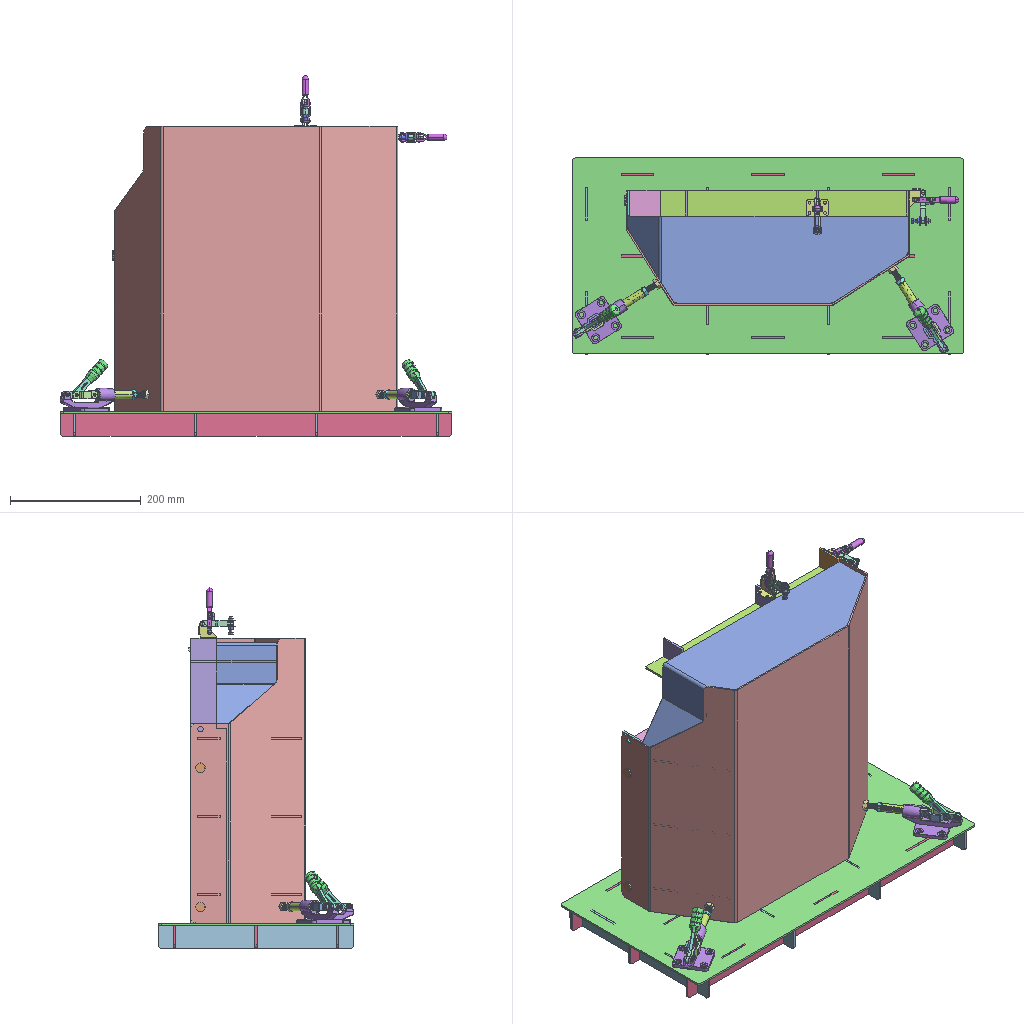Assembly | SolidWorks | 13 different items | 24 placed | box 600 x 300 x 552 mm
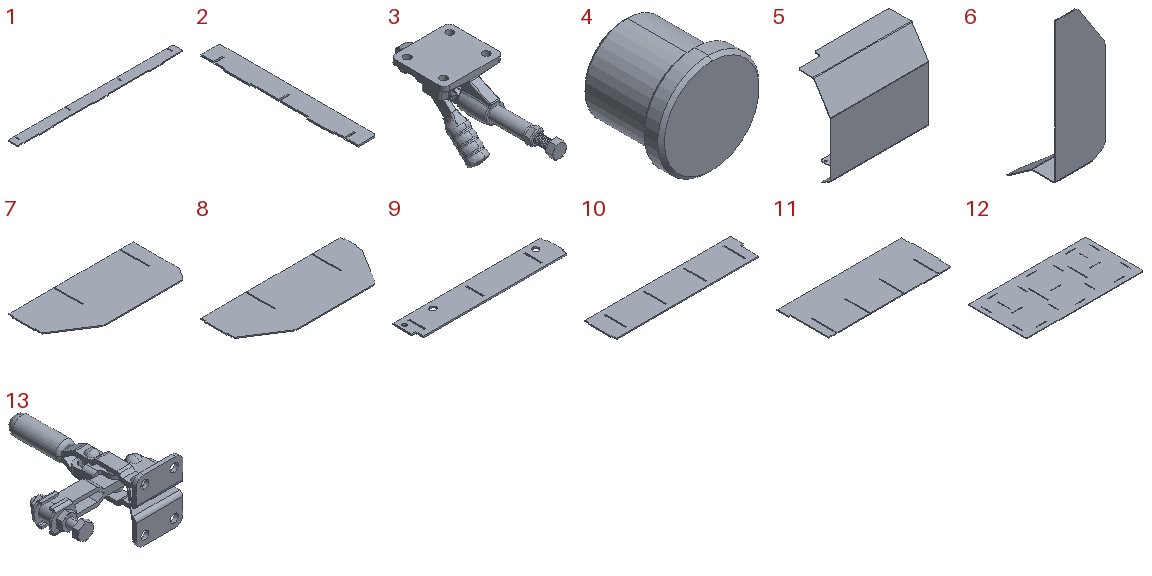Parts list (item | quantity | size | volume | features):
1 | x3 | 600 x 38 x 3.2 mm | 67879 mm3 | features FlatPattern 1, SMBaseFlange 1, SheetMetal 1
2 | x4 | 38 x 300 x 3.2 mm | 33980 mm3 | features FlatPattern 1, SMBaseFlange 1, SheetMetal 1
3 | x2 | 57.2 x 153.749 x 79.304 mm | 52807 mm3 | features BaseBody 11
4 | x2 | 15 x 13 x 15 mm | 1741 mm3 | features Chamfer 1, Revolution 1
5 | x1 | 436 x 176 x 434 mm | 633093 mm3 | features ICE 3, Fillet 1, FlatPattern 1, SMBaseFlange 1, SheetMetal 1
6 | x1 | 134 x 132 x 429.026 mm | 130634 mm3 | features Chamfer 1, FlatPattern 1, ICE 1, SMBaseFlange 1, SheetMetal 1
7 | x1 | 379.5 x 173.7 x 3.2 mm | 193629 mm3 | features FlatPattern 1, SMBaseFlange 1, SheetMetal 1
8 | x3 | 429 x 173.7 x 3.2 mm | 209173 mm3 | features FlatPattern 1, SMBaseFlange 1, SheetMetal 1
9 | x1 | 309 x 55 x 3.2 mm | 51735 mm3 | features FlatPattern 1, SMBaseFlange 1, SheetMetal 1
10 | x1 | 439 x 95 x 3.2 mm | 129037 mm3 | features FlatPattern 1, SMBaseFlange 1, SheetMetal 1
11 | x2 | 439 x 173.7 x 3.2 mm | 236184 mm3 | features FlatPattern 1, SMBaseFlange 1, SheetMetal 1
12 | x1 | 600 x 300 x 3.2 mm | 564155 mm3 | features FlatPattern 1, SMBaseFlange 1, SheetMetal 1
13 | x2 | 56.45 x 77.62 x 33.3 mm | 10418 mm3 | features BaseBody 5
Mates (type | each side: item.copy, entity, surface, feature):
DistanceDim | 6.1 face plane Base-Flange1 | 5.1 face plane Base-Flange1
Coincident | 5.1 face plane Base-Flange1 | 6.1 face plane Base-Flange1 | 2 times
InPlace | 7.1 plane | assembly plane
InPlace | 8.1 plane | assembly plane
InPlace | 5.1 face plane Base-Flange1 | 9.1 plane
InPlace | 5.1 face plane Base-Flange1 | 10.1 plane
InPlace | 11.1 plane | assembly plane
InPlace | 5.1 face plane Base-Flange1 | 12.1 plane
InPlace | 1.1 plane | assembly plane
InPlace | 2.1 plane | assembly plane
Coincident | 10.1 face plane Base-Flange1 | 13.1 face plane TC1-1 vertical flange-mount toggle clamp [TCS1-1].step-1/_TCS1-1(seat).step-1-solid1 | 3 times
Coincident | 5.1 face plane Base-Flange1 | 3.1 face plane
Coincident | 12.1 face plane Base-Flange1 | 3.1 face plane
DistanceDim | 3.1 face cylinder | 12.1 face plane Base-Flange1
Coincident | 5.1 face plane Base-Flange1 | 3.2 face plane
Coincident | 12.1 face plane Base-Flange1 | 3.2 face plane
DistanceDim | 3.2 face cylinder | 12.1 face plane Base-Flange1
Concentric | 5.1 face cylinder Cut-Extrude1 | 4.1 face cylinder Revolve1
Coincident | 5.1 face plane Base-Flange1 | 4.1 face plane Revolve1
Coincident | 11.2 face plane Base-Flange1 | 13.2 face plane TC1-1 vertical flange-mount toggle clamp [TCS1-1].step-1/_TCS1-1(seat).step-1-solid1 | 3 times